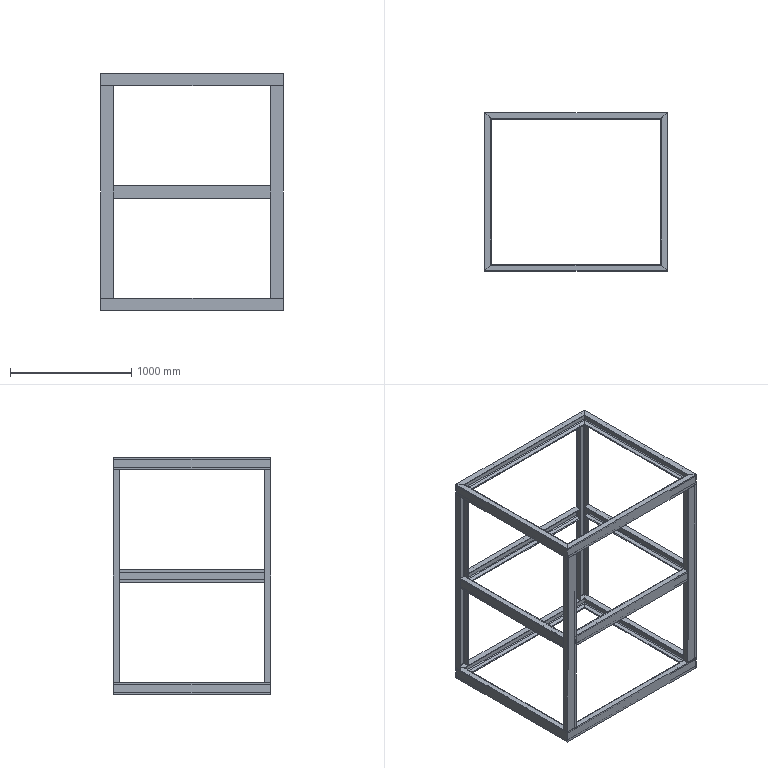Part | STEP file | Bracket 2XG(default_machined_) | 16 solids | 224 faces | box 1500 x 1300 x 1950 mm | volume 30079515 mm3 | plane 160 | cylinder 64 | commonest cylinder face diameters 9 x32 16 x32